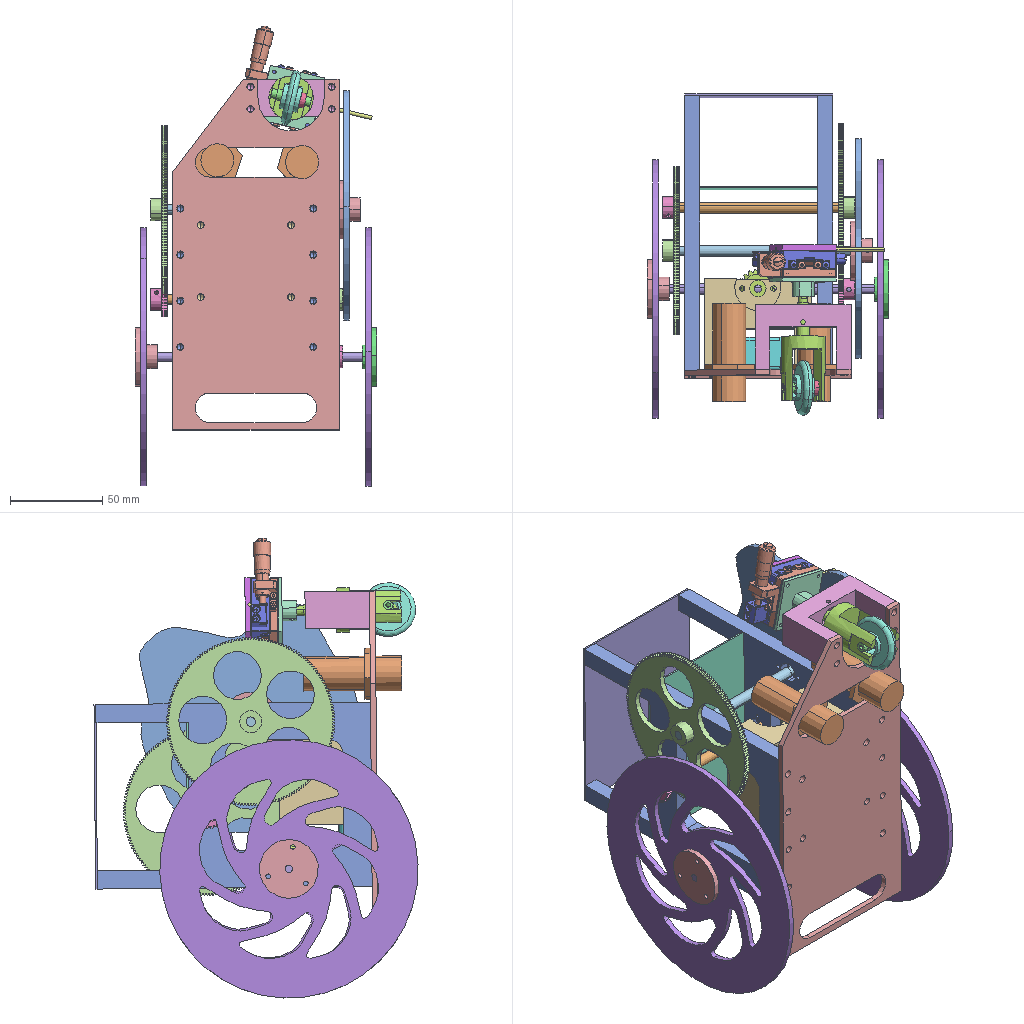Assembly | SolidWorks | 30 different items | 36 placed | box 131 x 176 x 249 mm
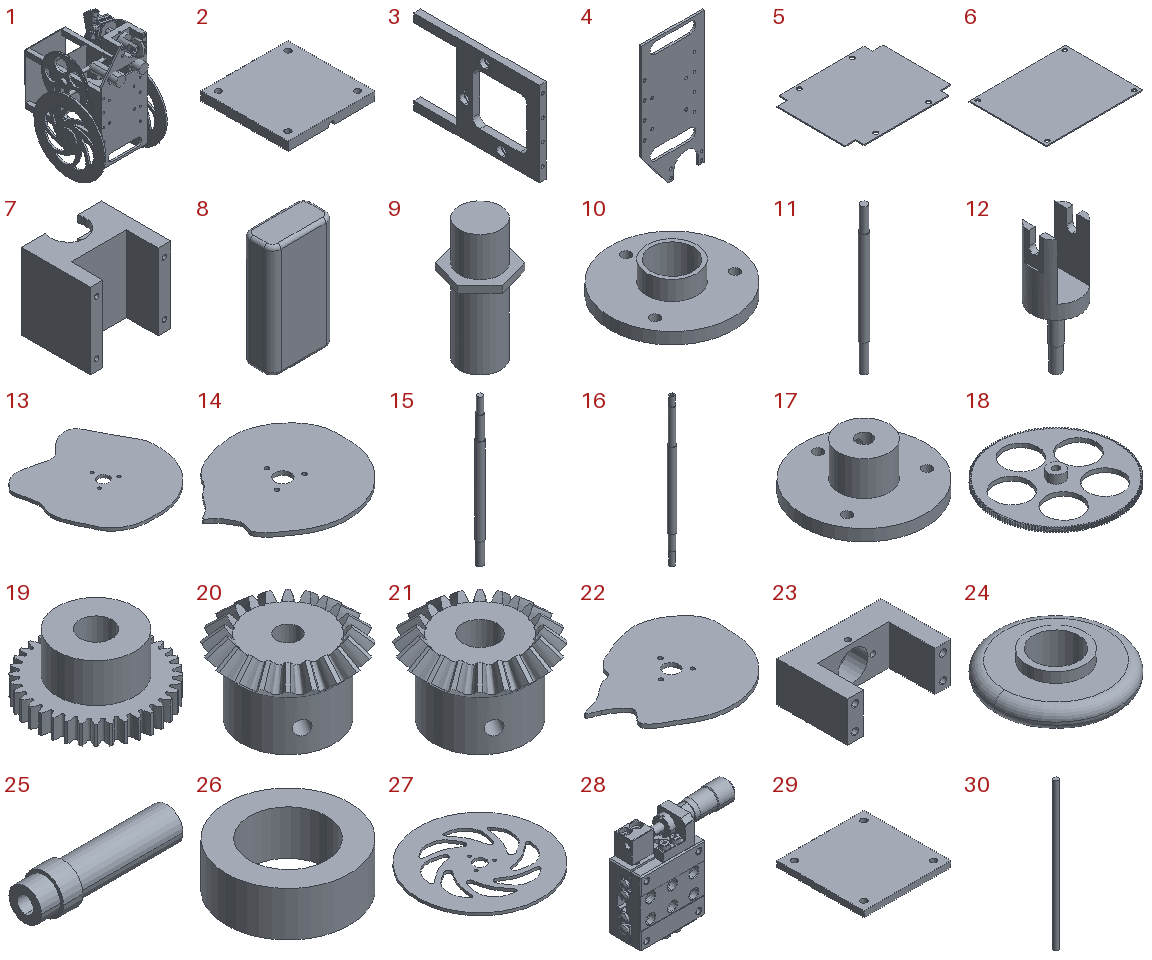Parts list (item | name | quantity | size | volume | features):
1 | (subassembly) | x1 | 131 x 175.611 x 249.309 mm | 497215 mm3 | features CompositeCurve 1, LayoutProfileFeature 1
2 | - | x1 | 30 x 30 x 3 mm | 2591 mm3 | features ICE 2, Extrusion 1
3 | - | x2 | 8 x 148.83 x 100 mm | 54028 mm3 | features HoleWzd 4, ICE 3, 3DProfileFeature 1, Extrusion 1, Fillet 1
4 | - | x1 | 90 x 3 x 190 mm | 39234 mm3 | features Extrusion 1, ICE 1
5 | - | x1 | 100 x 80 x 1 mm | 7630 mm3 | features Extrusion 1
6 | - | x1 | 100 x 80 x 1 mm | 7950 mm3 | features Extrusion 1
7 | - | x1 | 58 x 50 x 55 mm | 71255 mm3 | features ICE 4, Extrusion 1, HoleWzd 1
8 | - | x1 | 36 x 18 x 65 mm | 40559 mm3 | features Fillet 2, Extrusion 1
9 | - | x2 | 26.811 x 26.725 x 53 mm | 14220 mm3 | features Extrusion 1, ICE 1
10 | - | x1 | 32 x 32 x 8 mm | 2272 mm3 | features ICE 3, Extrusion 1, HoleWzd 1
11 | - | x1 | 6 x 6 x 104 mm | 2621 mm3 | features ICE 2, Extrusion 1
12 | - | x1 | 24 x 24 x 65.5 mm | 6275 mm3 | features ICE 7, Extrusion 1
13 | - | x1 | 118.036 x 124.021 x 3 mm | 33767 mm3 | features CurveInFile 1, Extrusion 1, ICE 1
14 | - | x1 | 106.214 x 95.117 x 3 mm | 21730 mm3 | features ICE 2, CurveInFile 1, Extrusion 1
15 | - | x1 | 6 x 6 x 113.5 mm | 2723 mm3 | features ICE 3, Extrusion 1
16 | - | x1 | 6 x 6 x 131 mm | 2988 mm3 | features ICE 4, 3DProfileFeature 1, Extrusion 1, HoleWzd 1
17 | - | x2 | 32 x 32 x 12 mm | 3390 mm3 | features ICE 3, HoleWzd 2, Extrusion 1
18 | - | x2 | 90.992 x 90.992 x 9 mm | 9929 mm3 | features ICE 3, 3DProfileFeature 1, CirPattern 1, HoleWzd 1, RefAxis 1, Revolution 1
19 | - | x2 | 18.957 x 18.957 x 9 mm | 1231 mm3 | features ICE 3, 3DProfileFeature 1, CirPattern 1, HoleWzd 1, RefAxis 1, Revolution 1
20 | - | x1 | 21.253 x 21.253 x 13.804 mm | 2568 mm3 | features 3DProfileFeature 9, ICE 2, BlendCut 1, CirPattern 1, CurveInFile 1, HoleWzd 1, RefAxis 1, RevCut 1, Revolution 1
21 | - | x1 | 21.253 x 21.253 x 13.804 mm | 2380 mm3 | features 3DProfileFeature 9, ICE 2, BlendCut 1, CirPattern 1, CurveInFile 1, HoleWzd 1, RefAxis 1, RevCut 1, Revolution 1
22 | - | x1 | 115.273 x 93.626 x 3 mm | 21562 mm3 | features ICE 2, CurveInFile 1, Extrusion 1
23 | - | x1 | 52 x 35 x 20 mm | 17449 mm3 | features HoleWzd 3, ICE 3, Extrusion 1
24 | - | x1 | 30 x 30 x 10 mm | 3110 mm3 | features ICE 2, Extrusion 1, Fillet 1
25 | - | x1 | 21.8 x 6 x 6 mm | 372.962 mm3 | features 3DProfileFeature 1, HoleWzd 1, Revolution 1
26 | - | x1 | 8 x 8 x 2.9 mm | 88.829 mm3 | features Extrusion 1
27 | - | x2 | 140 x 140 x 3 mm | 34568 mm3 | features Extrusion 1, ICE 1
28 | - | x1 | 51.773 x 15 x 49.6 mm | 14054 mm3 | features MBimport 1
29 | - | x1 | 30 x 30 x 10 mm | 2417 mm3 | features ICE 5, HoleWzd 2, Extrusion 1
30 | - | x1 | 2 x 2 x 60 mm | 188.496 mm3 | features Extrusion 1
Mates (type | each side: item.copy, entity, surface, feature):
Coincident | 4.1 face plane Boss-Extrude1 | 3.1 face plane Boss-Extrude1
Concentric | 4.1 face cylinder Cut-Extrude1 | 3.1 face cylinder M4 Tapped Hole1 | 2 times
Coincident | 4.1 face plane Boss-Extrude1 | 3.2 face plane Boss-Extrude1
Concentric | 4.1 face cylinder Cut-Extrude1 | 3.2 face cylinder M4 Tapped Hole1 | 2 times
Coincident | 4.1 face plane Boss-Extrude1 | 23.1 face plane Boss-Extrude1
Concentric | 4.1 face cylinder Cut-Extrude1 | 23.1 face cylinder M4 Tapped Hole1 | 2 times
Concentric | 12.1 face cylinder Boss-Extrude3 | 23.1 face cylinder Cut-Extrude5
Coincident | 12.1 face plane Boss-Extrude2 | 23.1 face plane Boss-Extrude1
Concentric | 12.1 face cylinder Cut-Extrude2 | 24.1 face cylinder Cut-Extrude1
Concentric | 3.1 face cylinder Cut-Extrude2 | 11.1 face cylinder Boss-Extrude2
Coincident | 3.1 face plane Cut-Extrude2 | 11.1 face plane Boss-Extrude2
Concentric | 3.2 face cylinder Cut-Extrude2 | 16.1 face cylinder Boss-Extrude2
Concentric | 3.1 face cylinder Cut-Extrude2 | 15.1 face cylinder Boss-Extrude2
Concentric | 12.1 face cylinder Cut-Extrude2 | 25.1 face cylinder Revolve1
Coincident | 12.1 face plane Cut-Extrude1 | 25.1 face plane Revolve1
Coincident | 24.1 face plane Boss-Extrude2 | 25.1 face plane Revolve1
Coincident | 12.1 face plane Cut-Extrude1 | 26.1 face plane Boss-Extrude1
Concentric | 25.1 face cylinder Revolve1 | 26.1 face cylinder Boss-Extrude1
Concentric | 12.1 face cylinder Boss-Extrude4 | 29.1 face cylinder Cut-Extrude3
Parallel | 12.1 face plane Cut-Extrude4 | 29.1 face plane Cut-Extrude5
Coincident | 12.1 face plane Boss-Extrude4 | 29.1 face plane Cut-Extrude3
Coincident | 29.1 face plane Boss-Extrude1 | 28.1 face plane LX30-L.stp
Concentric | 29.1 face cylinder M2.5 Tapped Hole1 | 28.1 face cylinder LX30-L.stp | 2 times
Coincident | 2.1 face plane Boss-Extrude1 | 28.1 face plane LX30-L.stp
Concentric | 2.1 face cylinder Cut-Extrude1 | 28.1 face cylinder LX30-L.stp | 2 times
Concentric | 30.1 face cylinder Boss-Extrude1 | 2.1 face cylinder Cut-Extrude2
Coincident | 30.1 face plane Boss-Extrude1 | 2.1 face plane Boss-Extrude1
Concentric | 16.1 face cylinder Boss-Extrude1 | 19.1 face cylinder Cut-Extrude2
Coincident | 18.1 face plane Boss-Extrude1 | 19.1 face plane Boss-Extrude1
Concentric | 11.1 face cylinder Boss-Extrude1 | 18.1 face cylinder Cut-Extrude2
Coincident | 11.1 face plane Boss-Extrude1 | 18.1 face plane Boss-Extrude1
Concentric | 11.1 face cylinder Boss-Extrude3 | 19.2 face cylinder Cut-Extrude2
Coincident | 3.1 face plane Cut-Extrude2 | 15.1 face plane Boss-Extrude2
Concentric | 15.1 face cylinder Boss-Extrude1 | 18.2 face cylinder Cut-Extrude2
Coincident | 18.2 face plane Large Spur Gear | 19.2 face plane Small Spur Gear
Coincident | 15.1 face plane Boss-Extrude1 | 18.2 face plane Boss-Extrude1
Concentric | 4.1 face cylinder Cut-Extrude1 | 7.1 face cylinder M4 Tapped Hole1 | 2 times
Coincident | 4.1 face plane Boss-Extrude1 | 7.1 face plane Boss-Extrude1
Coincident | 4.1 face plane Boss-Extrude1 | 8.1 face plane Boss-Extrude1
Concentric | 16.1 face cylinder Boss-Extrude4 | 10.1 face cylinder Cut-Extrude1
Concentric | 27.1 face cylinder Boss-Extrude1 | 10.1 face cylinder Boss-Extrude2
Concentric | 27.1 face cylinder Boss-Extrude1 | 10.1 face cylinder M3 Tapped Hole1
Coincident | 27.1 face plane Boss-Extrude1 | 10.1 face plane Boss-Extrude1
Coincident | 16.1 face plane Boss-Extrude4 | 10.1 face plane Boss-Extrude1
Concentric | 16.1 face cylinder Boss-Extrude5 | 17.1 face cylinder Cut-Extrude1
Coincident | 16.1 face plane Boss-Extrude5 | 17.1 face plane Boss-Extrude1
Concentric | 17.1 face cylinder Boss-Extrude2 | 27.2 face cylinder Boss-Extrude1
Concentric | 17.1 face cylinder M3 Tapped Hole6 | 27.2 face cylinder Boss-Extrude1
Coincident | 17.1 face plane Boss-Extrude1 | 27.2 face plane Boss-Extrude1
Concentric | 15.1 face cylinder Boss-Extrude4 | 17.2 face cylinder Cut-Extrude1
Coincident | 15.1 face plane Boss-Extrude3 | 17.2 face plane Boss-Extrude1
Concentric | 17.2 face cylinder Boss-Extrude2 | 13.1 face cylinder Cut-Extrude1
Coincident | 17.2 face plane Boss-Extrude1 | 13.1 face plane Boss-Extrude1
Concentric | 17.2 face cylinder M3 Tapped Hole6 | 13.1 face cylinder Cut-Extrude1
Coincident | 3.1 face plane Cut-Extrude2 | 16.1 face plane Boss-Extrude2
Tangent | 30.1 face cylinder Boss-Extrude1 | 13.1 edge
Concentric | 16.1 face cylinder Boss-Extrude2 | 21.1 face cylinder Cut-Extrude1
DistanceDim | 21.1 face plane Boss-Extrude1 | 3.2 face plane Boss-Extrude1
DistanceDim | 20.1 face plane Cut-Revolve2 | 16.1 face cylinder Boss-Extrude2
Coincident | 3.2 face plane Boss-Extrude1 | 5.1 face plane Boss-Extrude1
Coincident | 4.1 face plane Boss-Extrude1 | 9.1 face plane Boss-Extrude2
Concentric | 4.1 face cylinder Cut-Extrude1 | 9.1 face cylinder Boss-Extrude1
Coincident | 4.1 face plane Boss-Extrude1 | 9.2 face plane Boss-Extrude2
Tangent | 4.1 face plane Cut-Extrude1 | 9.2 face cylinder Boss-Extrude1
Concentric | 3.2 face cylinder M4 Tapped Hole6 | 5.1 face cylinder Boss-Extrude1 | 2 times
Concentric | 3.2 face cylinder M4 Tapped Hole5 | 6.1 face cylinder Boss-Extrude1 | 2 times
Coincident | 3.2 face plane Boss-Extrude2 | 6.1 face plane Boss-Extrude1